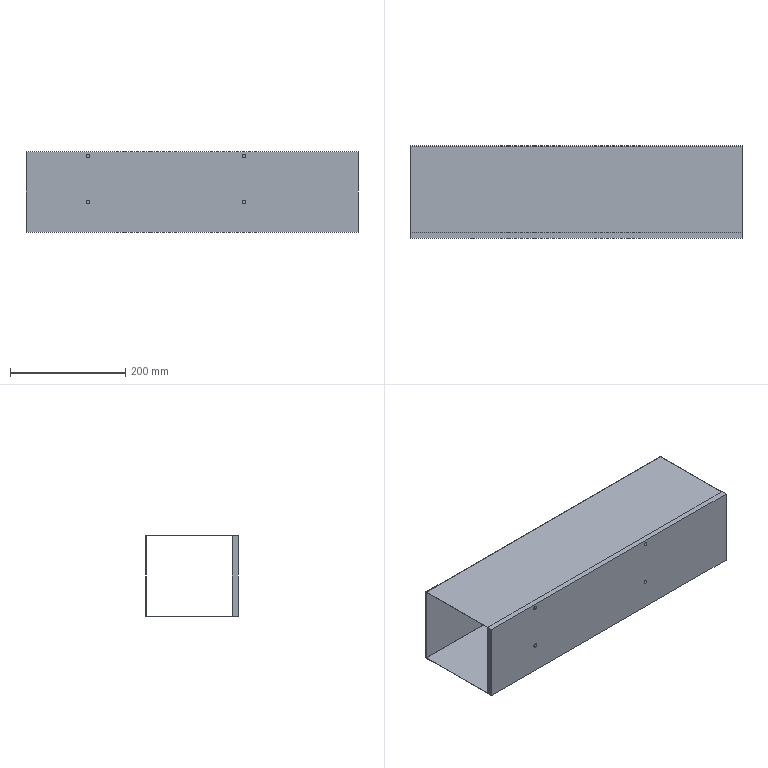Part | STEP file | 0245_Work-A | 1 solid | 18 faces | box 575 x 160 x 140 mm | volume 929885 mm3 | plane 10 | cylinder 8 | commonest cylinder face diameters 6.5 x8
STEP:
#1=CARTESIAN_POINT('',(0.,0.,0.));
#2=DIRECTION('',(0.,0.,1.));
#3=DIRECTION('',(1.,0.,0.));
#4=AXIS2_PLACEMENT_3D('',#1,#2,#3);
#5=CARTESIAN_POINT('',(377.5,0.,-84.25));
#6=VERTEX_POINT('',#5);
#7=CARTESIAN_POINT('',(377.5,10.,-84.25));
#8=VERTEX_POINT('',#7);
#9=CARTESIAN_POINT('',(377.5,10.,-84.25));
#10=DIRECTION('',(0.,1.,0.));
#11=VECTOR('',#10,1.);
#12=LINE('',#9,#11);
#13=CARTESIAN_POINT('',(377.5,10.,-87.5));
#14=DIRECTION('',(0.,1.,0.));
#15=DIRECTION('',(0.,0.,1.));
#16=AXIS2_PLACEMENT_3D('',#13,#14,#15);
#17=CYLINDRICAL_SURFACE('',#16,3.25);
#18=CARTESIAN_POINT('',(6.283,0.));
#19=DIRECTION('',(0.,1.));
#20=VECTOR('',#19,1.);
#21=LINE('',#18,#20);
#22=(GEOMETRIC_REPRESENTATION_CONTEXT(2)PARAMETRIC_REPRESENTATION_CONTEXT()REPRESENTATION_CONTEXT('',''));
#23=DEFINITIONAL_REPRESENTATION('',(#21),#22);
#24=PCURVE('',#17,#23);
#25=CARTESIAN_POINT('',(377.5,10.,-87.5));
#26=DIRECTION('',(0.,1.,0.));
#27=DIRECTION('',(0.,0.,1.));
#28=AXIS2_PLACEMENT_3D('',#25,#26,#27);
#29=CYLINDRICAL_SURFACE('',#28,3.25);
#30=CARTESIAN_POINT('',(0.,0.));
#31=DIRECTION('',(0.,1.));
#32=VECTOR('',#31,1.);
#33=LINE('',#30,#32);
#34=(GEOMETRIC_REPRESENTATION_CONTEXT(2)PARAMETRIC_REPRESENTATION_CONTEXT()REPRESENTATION_CONTEXT('',''));
#35=DEFINITIONAL_REPRESENTATION('',(#33),#34);
#36=PCURVE('',#29,#35);
#37=SURFACE_CURVE('',#12,(#24,#36),.PCURVE_S1.);
#38=EDGE_CURVE('',#6,#8,#37,.T.);
#39=ORIENTED_EDGE('',*,*,#38,.T.);
#40=CARTESIAN_POINT('',(377.5,10.,-90.75));
#41=VERTEX_POINT('',#40);
#42=CARTESIAN_POINT('',(377.5,10.,-87.5));
#43=DIRECTION('',(0.,1.,0.));
#44=DIRECTION('',(0.,0.,1.));
#45=AXIS2_PLACEMENT_3D('',#42,#43,#44);
#46=CIRCLE('',#45,3.25);
#47=CARTESIAN_POINT('',(0.,0.));
#48=DIRECTION('',(1.,0.));
#49=VECTOR('',#48,1.);
#50=LINE('',#47,#49);
#51=(GEOMETRIC_REPRESENTATION_CONTEXT(2)PARAMETRIC_REPRESENTATION_CONTEXT()REPRESENTATION_CONTEXT('',''));
#52=DEFINITIONAL_REPRESENTATION('',(#50),#51);
#53=PCURVE('',#17,#52);
#54=CARTESIAN_POINT('',(575.,10.,-0.5));
#55=DIRECTION('',(0.,1.,0.));
#56=DIRECTION('',(0.,0.,1.));
#57=AXIS2_PLACEMENT_3D('',#54,#55,#56);
#58=PLANE('',#57);
#59=CARTESIAN_POINT('',(-87.,-197.5));
#60=DIRECTION('',(1.,0.));
#61=AXIS2_PLACEMENT_2D('',#59,#60);
#62=CIRCLE('',#61,3.25);
#63=(GEOMETRIC_REPRESENTATION_CONTEXT(2)PARAMETRIC_REPRESENTATION_CONTEXT()REPRESENTATION_CONTEXT('',''));
#64=DEFINITIONAL_REPRESENTATION('',(#62),#63);
#65=PCURVE('',#58,#64);
#66=SURFACE_CURVE('',#46,(#53,#65),.PCURVE_S1.);
#67=EDGE_CURVE('',#41,#8,#66,.T.);
#68=ORIENTED_EDGE('',*,*,#67,.F.);
#69=CARTESIAN_POINT('',(377.5,0.,-90.75));
#70=VERTEX_POINT('',#69);
#71=CARTESIAN_POINT('',(377.5,10.,-90.75));
#72=DIRECTION('',(0.,1.,0.));
#73=VECTOR('',#72,1.);
#74=LINE('',#71,#73);
#75=CARTESIAN_POINT('',(3.142,0.));
#76=DIRECTION('',(0.,1.));
#77=VECTOR('',#76,1.);
#78=LINE('',#75,#77);
#79=(GEOMETRIC_REPRESENTATION_CONTEXT(2)PARAMETRIC_REPRESENTATION_CONTEXT()REPRESENTATION_CONTEXT('',''));
#80=DEFINITIONAL_REPRESENTATION('',(#78),#79);
#81=PCURVE('',#17,#80);
#82=CARTESIAN_POINT('',(3.142,0.));
#83=DIRECTION('',(0.,1.));
#84=VECTOR('',#83,1.);
#85=LINE('',#82,#84);
#86=(GEOMETRIC_REPRESENTATION_CONTEXT(2)PARAMETRIC_REPRESENTATION_CONTEXT()REPRESENTATION_CONTEXT('',''));
#87=DEFINITIONAL_REPRESENTATION('',(#85),#86);
#88=PCURVE('',#29,#87);
#89=SURFACE_CURVE('',#74,(#81,#88),.PCURVE_S1.);
#90=EDGE_CURVE('',#70,#41,#89,.T.);
#91=ORIENTED_EDGE('',*,*,#90,.F.);
#92=CARTESIAN_POINT('',(377.5,0.,-87.5));
#93=DIRECTION('',(0.,1.,0.));
#94=DIRECTION('',(0.,0.,1.));
#95=AXIS2_PLACEMENT_3D('',#92,#93,#94);
#96=CIRCLE('',#95,3.25);
#97=CARTESIAN_POINT('',(0.,-10.));
#98=DIRECTION('',(1.,0.));
#99=VECTOR('',#98,1.);
#100=LINE('',#97,#99);
#101=(GEOMETRIC_REPRESENTATION_CONTEXT(2)PARAMETRIC_REPRESENTATION_CONTEXT()REPRESENTATION_CONTEXT('',''));
#102=DEFINITIONAL_REPRESENTATION('',(#100),#101);
#103=PCURVE('',#17,#102);
#104=CARTESIAN_POINT('',(575.,0.,0.));
#105=DIRECTION('',(0.,1.,0.));
#106=DIRECTION('',(0.,0.,1.));
#107=AXIS2_PLACEMENT_3D('',#104,#105,#106);
#108=PLANE('',#107);
#109=CARTESIAN_POINT('',(-87.5,-197.5));
#110=DIRECTION('',(1.,0.));
#111=AXIS2_PLACEMENT_2D('',#109,#110);
#112=CIRCLE('',#111,3.25);
#113=(GEOMETRIC_REPRESENTATION_CONTEXT(2)PARAMETRIC_REPRESENTATION_CONTEXT()REPRESENTATION_CONTEXT('',''));
#114=DEFINITIONAL_REPRESENTATION('',(#112),#113);
#115=PCURVE('',#108,#114);
#116=SURFACE_CURVE('',#96,(#103,#115),.PCURVE_S1.);
#117=EDGE_CURVE('',#70,#6,#116,.T.);
#118=ORIENTED_EDGE('',*,*,#117,.T.);
#119=EDGE_LOOP('',(#39,#68,#91,#118));
#120=FACE_BOUND('',#119,.F.);
#121=ADVANCED_FACE('',(#120),#17,.F.);
#122=CARTESIAN_POINT('',(107.5,0.,-84.25));
#123=VERTEX_POINT('',#122);
#124=CARTESIAN_POINT('',(107.5,10.,-84.25));
#125=VERTEX_POINT('',#124);
#126=CARTESIAN_POINT('',(107.5,10.,-84.25));
#127=DIRECTION('',(0.,1.,0.));
#128=VECTOR('',#127,1.);
#129=LINE('',#126,#128);
#130=CARTESIAN_POINT('',(107.5,10.,-87.5));
#131=DIRECTION('',(0.,1.,0.));
#132=DIRECTION('',(0.,0.,1.));
#133=AXIS2_PLACEMENT_3D('',#130,#131,#132);
#134=CYLINDRICAL_SURFACE('',#133,3.25);
#135=CARTESIAN_POINT('',(6.283,0.));
#136=DIRECTION('',(0.,1.));
#137=VECTOR('',#136,1.);
#138=LINE('',#135,#137);
#139=(GEOMETRIC_REPRESENTATION_CONTEXT(2)PARAMETRIC_REPRESENTATION_CONTEXT()REPRESENTATION_CONTEXT('',''));
#140=DEFINITIONAL_REPRESENTATION('',(#138),#139);
#141=PCURVE('',#134,#140);
#142=CARTESIAN_POINT('',(107.5,10.,-87.5));
#143=DIRECTION('',(0.,1.,0.));
#144=DIRECTION('',(0.,0.,1.));
#145=AXIS2_PLACEMENT_3D('',#142,#143,#144);
#146=CYLINDRICAL_SURFACE('',#145,3.25);
#147=CARTESIAN_POINT('',(0.,0.));
#148=DIRECTION('',(0.,1.));
#149=VECTOR('',#148,1.);
#150=LINE('',#147,#149);
#151=(GEOMETRIC_REPRESENTATION_CONTEXT(2)PARAMETRIC_REPRESENTATION_CONTEXT()REPRESENTATION_CONTEXT('',''));
#152=DEFINITIONAL_REPRESENTATION('',(#150),#151);
#153=PCURVE('',#146,#152);
#154=SURFACE_CURVE('',#129,(#141,#153),.PCURVE_S1.);
#155=EDGE_CURVE('',#123,#125,#154,.T.);
#156=ORIENTED_EDGE('',*,*,#155,.T.);
#157=CARTESIAN_POINT('',(107.5,10.,-90.75));
#158=VERTEX_POINT('',#157);
#159=CARTESIAN_POINT('',(107.5,10.,-87.5));
#160=DIRECTION('',(0.,1.,0.));
#161=DIRECTION('',(0.,0.,1.));
#162=AXIS2_PLACEMENT_3D('',#159,#160,#161);
#163=CIRCLE('',#162,3.25);
#164=CARTESIAN_POINT('',(0.,0.));
#165=DIRECTION('',(1.,0.));
#166=VECTOR('',#165,1.);
#167=LINE('',#164,#166);
#168=(GEOMETRIC_REPRESENTATION_CONTEXT(2)PARAMETRIC_REPRESENTATION_CONTEXT()REPRESENTATION_CONTEXT('',''));
#169=DEFINITIONAL_REPRESENTATION('',(#167),#168);
#170=PCURVE('',#134,#169);
#171=CARTESIAN_POINT('',(-87.,-467.5));
#172=DIRECTION('',(1.,0.));
#173=AXIS2_PLACEMENT_2D('',#171,#172);
#174=CIRCLE('',#173,3.25);
#175=(GEOMETRIC_REPRESENTATION_CONTEXT(2)PARAMETRIC_REPRESENTATION_CONTEXT()REPRESENTATION_CONTEXT('',''));
#176=DEFINITIONAL_REPRESENTATION('',(#174),#175);
#177=PCURVE('',#58,#176);
#178=SURFACE_CURVE('',#163,(#170,#177),.PCURVE_S1.);
#179=EDGE_CURVE('',#158,#125,#178,.T.);
#180=ORIENTED_EDGE('',*,*,#179,.F.);
#181=CARTESIAN_POINT('',(107.5,0.,-90.75));
#182=VERTEX_POINT('',#181);
#183=CARTESIAN_POINT('',(107.5,10.,-90.75));
#184=DIRECTION('',(0.,1.,0.));
#185=VECTOR('',#184,1.);
#186=LINE('',#183,#185);
#187=CARTESIAN_POINT('',(3.142,0.));
#188=DIRECTION('',(0.,1.));
#189=VECTOR('',#188,1.);
#190=LINE('',#187,#189);
#191=(GEOMETRIC_REPRESENTATION_CONTEXT(2)PARAMETRIC_REPRESENTATION_CONTEXT()REPRESENTATION_CONTEXT('',''));
#192=DEFINITIONAL_REPRESENTATION('',(#190),#191);
#193=PCURVE('',#134,#192);
#194=CARTESIAN_POINT('',(3.142,0.));
#195=DIRECTION('',(0.,1.));
#196=VECTOR('',#195,1.);
#197=LINE('',#194,#196);
#198=(GEOMETRIC_REPRESENTATION_CONTEXT(2)PARAMETRIC_REPRESENTATION_CONTEXT()REPRESENTATION_CONTEXT('',''));
#199=DEFINITIONAL_REPRESENTATION('',(#197),#198);
#200=PCURVE('',#146,#199);
#201=SURFACE_CURVE('',#186,(#193,#200),.PCURVE_S1.);
#202=EDGE_CURVE('',#182,#158,#201,.T.);
#203=ORIENTED_EDGE('',*,*,#202,.F.);
#204=CARTESIAN_POINT('',(107.5,0.,-87.5));
#205=DIRECTION('',(0.,1.,0.));
#206=DIRECTION('',(0.,0.,1.));
#207=AXIS2_PLACEMENT_3D('',#204,#205,#206);
#208=CIRCLE('',#207,3.25);
#209=CARTESIAN_POINT('',(0.,-10.));
#210=DIRECTION('',(1.,0.));
#211=VECTOR('',#210,1.);
#212=LINE('',#209,#211);
#213=(GEOMETRIC_REPRESENTATION_CONTEXT(2)PARAMETRIC_REPRESENTATION_CONTEXT()REPRESENTATION_CONTEXT('',''));
#214=DEFINITIONAL_REPRESENTATION('',(#212),#213);
#215=PCURVE('',#134,#214);
#216=CARTESIAN_POINT('',(-87.5,-467.5));
#217=DIRECTION('',(1.,0.));
#218=AXIS2_PLACEMENT_2D('',#216,#217);
#219=CIRCLE('',#218,3.25);
#220=(GEOMETRIC_REPRESENTATION_CONTEXT(2)PARAMETRIC_REPRESENTATION_CONTEXT()REPRESENTATION_CONTEXT('',''));
#221=DEFINITIONAL_REPRESENTATION('',(#219),#220);
#222=PCURVE('',#108,#221);
#223=SURFACE_CURVE('',#208,(#215,#222),.PCURVE_S1.);
#224=EDGE_CURVE('',#182,#123,#223,.T.);
#225=ORIENTED_EDGE('',*,*,#224,.T.);
#226=EDGE_LOOP('',(#156,#180,#203,#225));
#227=FACE_BOUND('',#226,.F.);
#228=ADVANCED_FACE('',(#227),#134,.F.);
#229=CARTESIAN_POINT('',(377.5,0.,-4.25));
#230=VERTEX_POINT('',#229);
#231=CARTESIAN_POINT('',(377.5,10.,-4.25));
#232=VERTEX_POINT('',#231);
#233=CARTESIAN_POINT('',(377.5,10.,-4.25));
#234=DIRECTION('',(0.,1.,0.));
#235=VECTOR('',#234,1.);
#236=LINE('',#233,#235);
#237=CARTESIAN_POINT('',(377.5,10.,-7.5));
#238=DIRECTION('',(0.,1.,0.));
#239=DIRECTION('',(0.,0.,1.));
#240=AXIS2_PLACEMENT_3D('',#237,#238,#239);
#241=CYLINDRICAL_SURFACE('',#240,3.25);
#242=CARTESIAN_POINT('',(6.283,0.));
#243=DIRECTION('',(0.,1.));
#244=VECTOR('',#243,1.);
#245=LINE('',#242,#244);
#246=(GEOMETRIC_REPRESENTATION_CONTEXT(2)PARAMETRIC_REPRESENTATION_CONTEXT()REPRESENTATION_CONTEXT('',''));
#247=DEFINITIONAL_REPRESENTATION('',(#245),#246);
#248=PCURVE('',#241,#247);
#249=CARTESIAN_POINT('',(377.5,10.,-7.5));
#250=DIRECTION('',(0.,1.,0.));
#251=DIRECTION('',(0.,0.,1.));
#252=AXIS2_PLACEMENT_3D('',#249,#250,#251);
#253=CYLINDRICAL_SURFACE('',#252,3.25);
#254=CARTESIAN_POINT('',(0.,0.));
#255=DIRECTION('',(0.,1.));
#256=VECTOR('',#255,1.);
#257=LINE('',#254,#256);
#258=(GEOMETRIC_REPRESENTATION_CONTEXT(2)PARAMETRIC_REPRESENTATION_CONTEXT()REPRESENTATION_CONTEXT('',''));
#259=DEFINITIONAL_REPRESENTATION('',(#257),#258);
#260=PCURVE('',#253,#259);
#261=SURFACE_CURVE('',#236,(#248,#260),.PCURVE_S1.);
#262=EDGE_CURVE('',#230,#232,#261,.T.);
#263=ORIENTED_EDGE('',*,*,#262,.T.);
#264=CARTESIAN_POINT('',(377.5,10.,-10.75));
#265=VERTEX_POINT('',#264);
#266=CARTESIAN_POINT('',(377.5,10.,-7.5));
#267=DIRECTION('',(0.,1.,0.));
#268=DIRECTION('',(0.,0.,1.));
#269=AXIS2_PLACEMENT_3D('',#266,#267,#268);
#270=CIRCLE('',#269,3.25);
#271=CARTESIAN_POINT('',(0.,0.));
#272=DIRECTION('',(1.,0.));
#273=VECTOR('',#272,1.);
#274=LINE('',#271,#273);
#275=(GEOMETRIC_REPRESENTATION_CONTEXT(2)PARAMETRIC_REPRESENTATION_CONTEXT()REPRESENTATION_CONTEXT('',''));
#276=DEFINITIONAL_REPRESENTATION('',(#274),#275);
#277=PCURVE('',#241,#276);
#278=CARTESIAN_POINT('',(-7.,-197.5));
#279=DIRECTION('',(1.,0.));
#280=AXIS2_PLACEMENT_2D('',#278,#279);
#281=CIRCLE('',#280,3.25);
#282=(GEOMETRIC_REPRESENTATION_CONTEXT(2)PARAMETRIC_REPRESENTATION_CONTEXT()REPRESENTATION_CONTEXT('',''));
#283=DEFINITIONAL_REPRESENTATION('',(#281),#282);
#284=PCURVE('',#58,#283);
#285=SURFACE_CURVE('',#270,(#277,#284),.PCURVE_S1.);
#286=EDGE_CURVE('',#265,#232,#285,.T.);
#287=ORIENTED_EDGE('',*,*,#286,.F.);
#288=CARTESIAN_POINT('',(377.5,0.,-10.75));
#289=VERTEX_POINT('',#288);
#290=CARTESIAN_POINT('',(377.5,10.,-10.75));
#291=DIRECTION('',(0.,1.,0.));
#292=VECTOR('',#291,1.);
#293=LINE('',#290,#292);
#294=CARTESIAN_POINT('',(3.142,0.));
#295=DIRECTION('',(0.,1.));
#296=VECTOR('',#295,1.);
#297=LINE('',#294,#296);
#298=(GEOMETRIC_REPRESENTATION_CONTEXT(2)PARAMETRIC_REPRESENTATION_CONTEXT()REPRESENTATION_CONTEXT('',''));
#299=DEFINITIONAL_REPRESENTATION('',(#297),#298);
#300=PCURVE('',#241,#299);
#301=CARTESIAN_POINT('',(3.142,0.));
#302=DIRECTION('',(0.,1.));
#303=VECTOR('',#302,1.);
#304=LINE('',#301,#303);
#305=(GEOMETRIC_REPRESENTATION_CONTEXT(2)PARAMETRIC_REPRESENTATION_CONTEXT()REPRESENTATION_CONTEXT('',''));
#306=DEFINITIONAL_REPRESENTATION('',(#304),#305);
#307=PCURVE('',#253,#306);
#308=SURFACE_CURVE('',#293,(#300,#307),.PCURVE_S1.);
#309=EDGE_CURVE('',#289,#265,#308,.T.);
#310=ORIENTED_EDGE('',*,*,#309,.F.);
#311=CARTESIAN_POINT('',(377.5,0.,-7.5));
#312=DIRECTION('',(0.,1.,0.));
#313=DIRECTION('',(0.,0.,1.));
#314=AXIS2_PLACEMENT_3D('',#311,#312,#313);
#315=CIRCLE('',#314,3.25);
#316=CARTESIAN_POINT('',(0.,-10.));
#317=DIRECTION('',(1.,0.));
#318=VECTOR('',#317,1.);
#319=LINE('',#316,#318);
#320=(GEOMETRIC_REPRESENTATION_CONTEXT(2)PARAMETRIC_REPRESENTATION_CONTEXT()REPRESENTATION_CONTEXT('',''));
#321=DEFINITIONAL_REPRESENTATION('',(#319),#320);
#322=PCURVE('',#241,#321);
#323=CARTESIAN_POINT('',(-7.5,-197.5));
#324=DIRECTION('',(1.,0.));
#325=AXIS2_PLACEMENT_2D('',#323,#324);
#326=CIRCLE('',#325,3.25);
#327=(GEOMETRIC_REPRESENTATION_CONTEXT(2)PARAMETRIC_REPRESENTATION_CONTEXT()REPRESENTATION_CONTEXT('',''));
#328=DEFINITIONAL_REPRESENTATION('',(#326),#327);
#329=PCURVE('',#108,#328);
#330=SURFACE_CURVE('',#315,(#322,#329),.PCURVE_S1.);
#331=EDGE_CURVE('',#289,#230,#330,.T.);
#332=ORIENTED_EDGE('',*,*,#331,.T.);
#333=EDGE_LOOP('',(#263,#287,#310,#332));
#334=FACE_BOUND('',#333,.F.);
#335=ADVANCED_FACE('',(#334),#241,.F.);
#336=CARTESIAN_POINT('',(107.5,0.,-4.25));
#337=VERTEX_POINT('',#336);
#338=CARTESIAN_POINT('',(107.5,10.,-4.25));
#339=VERTEX_POINT('',#338);
#340=CARTESIAN_POINT('',(107.5,10.,-4.25));
#341=DIRECTION('',(0.,1.,0.));
#342=VECTOR('',#341,1.);
#343=LINE('',#340,#342);
#344=CARTESIAN_POINT('',(107.5,10.,-7.5));
#345=DIRECTION('',(0.,1.,0.));
#346=DIRECTION('',(0.,0.,1.));
#347=AXIS2_PLACEMENT_3D('',#344,#345,#346);
#348=CYLINDRICAL_SURFACE('',#347,3.25);
#349=CARTESIAN_POINT('',(6.283,0.));
#350=DIRECTION('',(0.,1.));
#351=VECTOR('',#350,1.);
#352=LINE('',#349,#351);
#353=(GEOMETRIC_REPRESENTATION_CONTEXT(2)PARAMETRIC_REPRESENTATION_CONTEXT()REPRESENTATION_CONTEXT('',''));
#354=DEFINITIONAL_REPRESENTATION('',(#352),#353);
#355=PCURVE('',#348,#354);
#356=CARTESIAN_POINT('',(107.5,10.,-7.5));
#357=DIRECTION('',(0.,1.,0.));
#358=DIRECTION('',(0.,0.,1.));
#359=AXIS2_PLACEMENT_3D('',#356,#357,#358);
#360=CYLINDRICAL_SURFACE('',#359,3.25);
#361=CARTESIAN_POINT('',(0.,0.));
#362=DIRECTION('',(0.,1.));
#363=VECTOR('',#362,1.);
#364=LINE('',#361,#363);
#365=(GEOMETRIC_REPRESENTATION_CONTEXT(2)PARAMETRIC_REPRESENTATION_CONTEXT()REPRESENTATION_CONTEXT('',''));
#366=DEFINITIONAL_REPRESENTATION('',(#364),#365);
#367=PCURVE('',#360,#366);
#368=SURFACE_CURVE('',#343,(#355,#367),.PCURVE_S1.);
#369=EDGE_CURVE('',#337,#339,#368,.T.);
#370=ORIENTED_EDGE('',*,*,#369,.T.);
#371=CARTESIAN_POINT('',(107.5,10.,-10.75));
#372=VERTEX_POINT('',#371);
#373=CARTESIAN_POINT('',(107.5,10.,-7.5));
#374=DIRECTION('',(0.,1.,0.));
#375=DIRECTION('',(0.,0.,1.));
#376=AXIS2_PLACEMENT_3D('',#373,#374,#375);
#377=CIRCLE('',#376,3.25);
#378=CARTESIAN_POINT('',(0.,0.));
#379=DIRECTION('',(1.,0.));
#380=VECTOR('',#379,1.);
#381=LINE('',#378,#380);
#382=(GEOMETRIC_REPRESENTATION_CONTEXT(2)PARAMETRIC_REPRESENTATION_CONTEXT()REPRESENTATION_CONTEXT('',''));
#383=DEFINITIONAL_REPRESENTATION('',(#381),#382);
#384=PCURVE('',#348,#383);
#385=CARTESIAN_POINT('',(-7.,-467.5));
#386=DIRECTION('',(1.,0.));
#387=AXIS2_PLACEMENT_2D('',#385,#386);
#388=CIRCLE('',#387,3.25);
#389=(GEOMETRIC_REPRESENTATION_CONTEXT(2)PARAMETRIC_REPRESENTATION_CONTEXT()REPRESENTATION_CONTEXT('',''));
#390=DEFINITIONAL_REPRESENTATION('',(#388),#389);
#391=PCURVE('',#58,#390);
#392=SURFACE_CURVE('',#377,(#384,#391),.PCURVE_S1.);
#393=EDGE_CURVE('',#372,#339,#392,.T.);
#394=ORIENTED_EDGE('',*,*,#393,.F.);
#395=CARTESIAN_POINT('',(107.5,0.,-10.75));
#396=VERTEX_POINT('',#395);
#397=CARTESIAN_POINT('',(107.5,10.,-10.75));
#398=DIRECTION('',(0.,1.,0.));
#399=VECTOR('',#398,1.);
#400=LINE('',#397,#399);
#401=CARTESIAN_POINT('',(3.142,0.));
#402=DIRECTION('',(0.,1.));
#403=VECTOR('',#402,1.);
#404=LINE('',#401,#403);
#405=(GEOMETRIC_REPRESENTATION_CONTEXT(2)PARAMETRIC_REPRESENTATION_CONTEXT()REPRESENTATION_CONTEXT('',''));
#406=DEFINITIONAL_REPRESENTATION('',(#404),#405);
#407=PCURVE('',#348,#406);
#408=CARTESIAN_POINT('',(3.142,0.));
#409=DIRECTION('',(0.,1.));
#410=VECTOR('',#409,1.);
#411=LINE('',#408,#410);
#412=(GEOMETRIC_REPRESENTATION_CONTEXT(2)PARAMETRIC_REPRESENTATION_CONTEXT()REPRESENTATION_CONTEXT('',''));
#413=DEFINITIONAL_REPRESENTATION('',(#411),#412);
#414=PCURVE('',#360,#413);
#415=SURFACE_CURVE('',#400,(#407,#414),.PCURVE_S1.);
#416=EDGE_CURVE('',#396,#372,#415,.T.);
#417=ORIENTED_EDGE('',*,*,#416,.F.);
#418=CARTESIAN_POINT('',(107.5,0.,-7.5));
#419=DIRECTION('',(0.,1.,0.));
#420=DIRECTION('',(0.,0.,1.));
#421=AXIS2_PLACEMENT_3D('',#418,#419,#420);
#422=CIRCLE('',#421,3.25);
#423=CARTESIAN_POINT('',(0.,-10.));
#424=DIRECTION('',(1.,0.));
#425=VECTOR('',#424,1.);
#426=LINE('',#423,#425);
#427=(GEOMETRIC_REPRESENTATION_CONTEXT(2)PARAMETRIC_REPRESENTATION_CONTEXT()REPRESENTATION_CONTEXT('',''));
#428=DEFINITIONAL_REPRESENTATION('',(#426),#427);
#429=PCURVE('',#348,#428);
#430=CARTESIAN_POINT('',(-7.5,-467.5));
#431=DIRECTION('',(1.,0.));
#432=AXIS2_PLACEMENT_2D('',#430,#431);
#433=CIRCLE('',#432,3.25);
#434=(GEOMETRIC_REPRESENTATION_CONTEXT(2)PARAMETRIC_REPRESENTATION_CONTEXT()REPRESENTATION_CONTEXT('',''));
#435=DEFINITIONAL_REPRESENTATION('',(#433),#434);
#436=PCURVE('',#108,#435);
#437=SURFACE_CURVE('',#422,(#429,#436),.PCURVE_S1.);
#438=EDGE_CURVE('',#396,#337,#437,.T.);
#439=ORIENTED_EDGE('',*,*,#438,.T.);
#440=EDGE_LOOP('',(#370,#394,#417,#439));
#441=FACE_BOUND('',#440,.F.);
#442=ADVANCED_FACE('',(#441),#348,.F.);
#443=CARTESIAN_POINT('',(575.,160.,0.));
#444=VERTEX_POINT('',#443);
#445=CARTESIAN_POINT('',(575.,0.,0.));
#446=VERTEX_POINT('',#445);
#447=CARTESIAN_POINT('',(575.,0.,0.));
#448=DIRECTION('',(0.,-1.,0.));
#449=VECTOR('',#448,1.);
#450=LINE('',#447,#449);
#451=CARTESIAN_POINT('',(575.,160.,0.));
#452=DIRECTION('',(-1.,0.,0.));
#453=DIRECTION('',(0.,0.,1.));
#454=AXIS2_PLACEMENT_3D('',#451,#452,#453);
#455=PLANE('',#454);
#456=CARTESIAN_POINT('',(0.,-160.));
#457=DIRECTION('',(0.,-1.));
#458=VECTOR('',#457,1.);
#459=LINE('',#456,#458);
#460=(GEOMETRIC_REPRESENTATION_CONTEXT(2)PARAMETRIC_REPRESENTATION_CONTEXT()REPRESENTATION_CONTEXT('',''));
#461=DEFINITIONAL_REPRESENTATION('',(#459),#460);
#462=PCURVE('',#455,#461);
#463=CARTESIAN_POINT('',(575.,0.,0.));
#464=DIRECTION('',(0.,0.,-1.));
#465=DIRECTION('',(-1.,0.,0.));
#466=AXIS2_PLACEMENT_3D('',#463,#464,#465);
#467=PLANE('',#466);
#468=CARTESIAN_POINT('',(0.,0.));
#469=DIRECTION('',(0.,-1.));
#470=VECTOR('',#469,1.);
#471=LINE('',#468,#470);
#472=(GEOMETRIC_REPRESENTATION_CONTEXT(2)PARAMETRIC_REPRESENTATION_CONTEXT()REPRESENTATION_CONTEXT('',''));
#473=DEFINITIONAL_REPRESENTATION('',(#471),#472);
#474=PCURVE('',#467,#473);
#475=SURFACE_CURVE('',#450,(#462,#474),.PCURVE_S1.);
#476=EDGE_CURVE('',#444,#446,#475,.T.);
#477=ORIENTED_EDGE('',*,*,#476,.T.);
#478=CARTESIAN_POINT('',(575.,0.,-140.));
#479=VERTEX_POINT('',#478);
#480=CARTESIAN_POINT('',(575.,0.,0.));
#481=DIRECTION('',(0.,0.,-1.));
#482=VECTOR('',#481,1.);
#483=LINE('',#480,#482);
#484=CARTESIAN_POINT('',(0.,-160.));
#485=DIRECTION('',(-1.,0.));
#486=VECTOR('',#485,1.);
#487=LINE('',#484,#486);
#488=(GEOMETRIC_REPRESENTATION_CONTEXT(2)PARAMETRIC_REPRESENTATION_CONTEXT()REPRESENTATION_CONTEXT('',''));
#489=DEFINITIONAL_REPRESENTATION('',(#487),#488);
#490=PCURVE('',#455,#489);
#491=CARTESIAN_POINT('',(0.,0.));
#492=DIRECTION('',(-1.,0.));
#493=VECTOR('',#492,1.);
#494=LINE('',#491,#493);
#495=(GEOMETRIC_REPRESENTATION_CONTEXT(2)PARAMETRIC_REPRESENTATION_CONTEXT()REPRESENTATION_CONTEXT('',''));
#496=DEFINITIONAL_REPRESENTATION('',(#494),#495);
#497=PCURVE('',#108,#496);
#498=SURFACE_CURVE('',#483,(#490,#497),.PCURVE_S1.);
#499=EDGE_CURVE('',#446,#479,#498,.T.);
#500=ORIENTED_EDGE('',*,*,#499,.T.);
#501=CARTESIAN_POINT('',(575.,160.,-140.));
#502=VERTEX_POINT('',#501);
#503=CARTESIAN_POINT('',(575.,0.,-140.));
#504=DIRECTION('',(0.,1.,0.));
#505=VECTOR('',#504,1.);
#506=LINE('',#503,#505);
#507=CARTESIAN_POINT('',(-140.,-160.));
#508=DIRECTION('',(0.,1.));
#509=VECTOR('',#508,1.);
#510=LINE('',#507,#509);
#511=(GEOMETRIC_REPRESENTATION_CONTEXT(2)PARAMETRIC_REPRESENTATION_CONTEXT()REPRESENTATION_CONTEXT('',''));
#512=DEFINITIONAL_REPRESENTATION('',(#510),#511);
#513=PCURVE('',#455,#512);
#514=CARTESIAN_POINT('',(575.,0.,-140.));
#515=DIRECTION('',(0.,0.,1.));
#516=DIRECTION('',(1.,0.,0.));
#517=AXIS2_PLACEMENT_3D('',#514,#515,#516);
#518=PLANE('',#517);
#519=CARTESIAN_POINT('',(0.,0.));
#520=DIRECTION('',(0.,1.));
#521=VECTOR('',#520,1.);
#522=LINE('',#519,#521);
#523=(GEOMETRIC_REPRESENTATION_CONTEXT(2)PARAMETRIC_REPRESENTATION_CONTEXT()REPRESENTATION_CONTEXT('',''));
#524=DEFINITIONAL_REPRESENTATION('',(#522),#523);
#525=PCURVE('',#518,#524);
#526=SURFACE_CURVE('',#506,(#513,#525),.PCURVE_S1.);
#527=EDGE_CURVE('',#479,#502,#526,.T.);
#528=ORIENTED_EDGE('',*,*,#527,.T.);
#529=CARTESIAN_POINT('',(575.,160.,0.));
#530=DIRECTION('',(0.,0.,1.));
#531=VECTOR('',#530,1.);
#532=LINE('',#529,#531);
#533=CARTESIAN_POINT('',(0.,0.));
#534=DIRECTION('',(1.,0.));
#535=VECTOR('',#534,1.);
#536=LINE('',#533,#535);
#537=(GEOMETRIC_REPRESENTATION_CONTEXT(2)PARAMETRIC_REPRESENTATION_CONTEXT()REPRESENTATION_CONTEXT('',''));
#538=DEFINITIONAL_REPRESENTATION('',(#536),#537);
#539=PCURVE('',#455,#538);
#540=CARTESIAN_POINT('',(575.,160.,0.));
#541=DIRECTION('',(0.,-1.,0.));
#542=DIRECTION('',(0.,0.,-1.));
#543=AXIS2_PLACEMENT_3D('',#540,#541,#542);
#544=PLANE('',#543);
#545=CARTESIAN_POINT('',(0.,0.));
#546=DIRECTION('',(-1.,0.));
#547=VECTOR('',#546,1.);
#548=LINE('',#545,#547);
#549=(GEOMETRIC_REPRESENTATION_CONTEXT(2)PARAMETRIC_REPRESENTATION_CONTEXT()REPRESENTATION_CONTEXT('',''));
#550=DEFINITIONAL_REPRESENTATION('',(#548),#549);
#551=PCURVE('',#544,#550);
#552=SURFACE_CURVE('',#532,(#539,#551),.PCURVE_S1.);
#553=EDGE_CURVE('',#502,#444,#552,.T.);
#554=ORIENTED_EDGE('',*,*,#553,.T.);
#555=EDGE_LOOP('',(#477,#500,#528,#554));
#556=FACE_BOUND('',#555,.T.);
#557=CARTESIAN_POINT('',(575.,159.5,-0.5));
#558=VERTEX_POINT('',#557);
#559=CARTESIAN_POINT('',(575.,10.,-0.5));
#560=VERTEX_POINT('',#559);
#561=CARTESIAN_POINT('',(575.,10.,-0.5));
#562=DIRECTION('',(0.,-1.,0.));
#563=VECTOR('',#562,1.);
#564=LINE('',#561,#563);
#565=CARTESIAN_POINT('',(-0.5,-150.));
#566=DIRECTION('',(0.,-1.));
#567=VECTOR('',#566,1.);
#568=LINE('',#565,#567);
#569=(GEOMETRIC_REPRESENTATION_CONTEXT(2)PARAMETRIC_REPRESENTATION_CONTEXT()REPRESENTATION_CONTEXT('',''));
#570=DEFINITIONAL_REPRESENTATION('',(#568),#569);
#571=PCURVE('',#455,#570);
#572=CARTESIAN_POINT('',(575.,10.,-0.5));
#573=DIRECTION('',(0.,0.,-1.));
#574=DIRECTION('',(-1.,0.,0.));
#575=AXIS2_PLACEMENT_3D('',#572,#573,#574);
#576=PLANE('',#575);
#577=CARTESIAN_POINT('',(0.,0.));
#578=DIRECTION('',(0.,-1.));
#579=VECTOR('',#578,1.);
#580=LINE('',#577,#579);
#581=(GEOMETRIC_REPRESENTATION_CONTEXT(2)PARAMETRIC_REPRESENTATION_CONTEXT()REPRESENTATION_CONTEXT('',''));
#582=DEFINITIONAL_REPRESENTATION('',(#580),#581);
#583=PCURVE('',#576,#582);
#584=SURFACE_CURVE('',#564,(#571,#583),.PCURVE_S1.);
#585=EDGE_CURVE('',#558,#560,#584,.T.);
#586=ORIENTED_EDGE('',*,*,#585,.F.);
#587=CARTESIAN_POINT('',(575.,159.5,-139.5));
#588=VERTEX_POINT('',#587);
#589=CARTESIAN_POINT('',(575.,159.5,-0.5));
#590=DIRECTION('',(0.,0.,1.));
#591=VECTOR('',#590,1.);
#592=LINE('',#589,#591);
#593=CARTESIAN_POINT('',(-0.5,-0.5));
#594=DIRECTION('',(1.,0.));
#595=VECTOR('',#594,1.);
#596=LINE('',#593,#595);
#597=(GEOMETRIC_REPRESENTATION_CONTEXT(2)PARAMETRIC_REPRESENTATION_CONTEXT()REPRESENTATION_CONTEXT('',''));
#598=DEFINITIONAL_REPRESENTATION('',(#596),#597);
#599=PCURVE('',#455,#598);
#600=CARTESIAN_POINT('',(575.,159.5,-0.5));
#601=DIRECTION('',(0.,-1.,0.));
#602=DIRECTION('',(0.,0.,-1.));
#603=AXIS2_PLACEMENT_3D('',#600,#601,#602);
#604=PLANE('',#603);
#605=CARTESIAN_POINT('',(0.,0.));
#606=DIRECTION('',(-1.,0.));
#607=VECTOR('',#606,1.);
#608=LINE('',#605,#607);
#609=(GEOMETRIC_REPRESENTATION_CONTEXT(2)PARAMETRIC_REPRESENTATION_CONTEXT()REPRESENTATION_CONTEXT('',''));
#610=DEFINITIONAL_REPRESENTATION('',(#608),#609);
#611=PCURVE('',#604,#610);
#612=SURFACE_CURVE('',#592,(#599,#611),.PCURVE_S1.);
#613=EDGE_CURVE('',#588,#558,#612,.T.);
#614=ORIENTED_EDGE('',*,*,#613,.F.);
#615=CARTESIAN_POINT('',(575.,10.,-139.5));
#616=VERTEX_POINT('',#615);
#617=CARTESIAN_POINT('',(575.,10.,-139.5));
#618=DIRECTION('',(0.,1.,0.));
#619=VECTOR('',#618,1.);
#620=LINE('',#617,#619);
#621=CARTESIAN_POINT('',(-139.5,-150.));
#622=DIRECTION('',(0.,1.));
#623=VECTOR('',#622,1.);
#624=LINE('',#621,#623);
#625=(GEOMETRIC_REPRESENTATION_CONTEXT(2)PARAMETRIC_REPRESENTATION_CONTEXT()REPRESENTATION_CONTEXT('',''));
#626=DEFINITIONAL_REPRESENTATION('',(#624),#625);
#627=PCURVE('',#455,#626);
#628=CARTESIAN_POINT('',(575.,10.,-139.5));
#629=DIRECTION('',(0.,0.,1.));
#630=DIRECTION('',(1.,0.,0.));
#631=AXIS2_PLACEMENT_3D('',#628,#629,#630);
#632=PLANE('',#631);
#633=CARTESIAN_POINT('',(0.,0.));
#634=DIRECTION('',(0.,1.));
#635=VECTOR('',#634,1.);
#636=LINE('',#633,#635);
#637=(GEOMETRIC_REPRESENTATION_CONTEXT(2)PARAMETRIC_REPRESENTATION_CONTEXT()REPRESENTATION_CONTEXT('',''));
#638=DEFINITIONAL_REPRESENTATION('',(#636),#637);
#639=PCURVE('',#632,#638);
#640=SURFACE_CURVE('',#620,(#627,#639),.PCURVE_S1.);
#641=EDGE_CURVE('',#616,#588,#640,.T.);
#642=ORIENTED_EDGE('',*,*,#641,.F.);
#643=CARTESIAN_POINT('',(575.,10.,-0.5));
#644=DIRECTION('',(0.,0.,-1.));
#645=VECTOR('',#644,1.);
#646=LINE('',#643,#645);
#647=CARTESIAN_POINT('',(-0.5,-150.));
#648=DIRECTION('',(-1.,0.));
#649=VECTOR('',#648,1.);
#650=LINE('',#647,#649);
#651=(GEOMETRIC_REPRESENTATION_CONTEXT(2)PARAMETRIC_REPRESENTATION_CONTEXT()REPRESENTATION_CONTEXT('',''));
#652=DEFINITIONAL_REPRESENTATION('',(#650),#651);
#653=PCURVE('',#455,#652);
#654=CARTESIAN_POINT('',(0.,0.));
#655=DIRECTION('',(-1.,0.));
#656=VECTOR('',#655,1.);
#657=LINE('',#654,#656);
#658=(GEOMETRIC_REPRESENTATION_CONTEXT(2)PARAMETRIC_REPRESENTATION_CONTEXT()REPRESENTATION_CONTEXT('',''));
#659=DEFINITIONAL_REPRESENTATION('',(#657),#658);
#660=PCURVE('',#58,#659);
#661=SURFACE_CURVE('',#646,(#653,#660),.PCURVE_S1.);
#662=EDGE_CURVE('',#560,#616,#661,.T.);
#663=ORIENTED_EDGE('',*,*,#662,.F.);
#664=EDGE_LOOP('',(#586,#614,#642,#663));
#665=FACE_BOUND('',#664,.T.);
#666=ADVANCED_FACE('',(#556,#665),#455,.F.);
#667=CARTESIAN_POINT('',(0.,160.,0.));
#668=VERTEX_POINT('',#667);
#669=CARTESIAN_POINT('',(0.,0.,0.));
#670=VERTEX_POINT('',#669);
#671=CARTESIAN_POINT('',(0.,0.,0.));
#672=DIRECTION('',(0.,-1.,0.));
#673=VECTOR('',#672,1.);
#674=LINE('',#671,#673);
#675=CARTESIAN_POINT('',(0.,160.,0.));
#676=DIRECTION('',(-1.,0.,0.));
#677=DIRECTION('',(0.,0.,1.));
#678=AXIS2_PLACEMENT_3D('',#675,#676,#677);
#679=PLANE('',#678);
#680=CARTESIAN_POINT('',(0.,-160.));
#681=DIRECTION('',(0.,-1.));
#682=VECTOR('',#681,1.);
#683=LINE('',#680,#682);
#684=(GEOMETRIC_REPRESENTATION_CONTEXT(2)PARAMETRIC_REPRESENTATION_CONTEXT()REPRESENTATION_CONTEXT('',''));
#685=DEFINITIONAL_REPRESENTATION('',(#683),#684);
#686=PCURVE('',#679,#685);
#687=CARTESIAN_POINT('',(575.,0.));
#688=DIRECTION('',(0.,-1.));
#689=VECTOR('',#688,1.);
#690=LINE('',#687,#689);
#691=(GEOMETRIC_REPRESENTATION_CONTEXT(2)PARAMETRIC_REPRESENTATION_CONTEXT()REPRESENTATION_CONTEXT('',''));
#692=DEFINITIONAL_REPRESENTATION('',(#690),#691);
#693=PCURVE('',#467,#692);
#694=SURFACE_CURVE('',#674,(#686,#693),.PCURVE_S1.);
#695=EDGE_CURVE('',#668,#670,#694,.T.);
#696=ORIENTED_EDGE('',*,*,#695,.F.);
#697=CARTESIAN_POINT('',(0.,160.,-140.));
#698=VERTEX_POINT('',#697);
#699=CARTESIAN_POINT('',(0.,160.,0.));
#700=DIRECTION('',(0.,0.,1.));
#701=VECTOR('',#700,1.);
#702=LINE('',#699,#701);
#703=CARTESIAN_POINT('',(0.,0.));
#704=DIRECTION('',(1.,0.));
#705=VECTOR('',#704,1.);
#706=LINE('',#703,#705);
#707=(GEOMETRIC_REPRESENTATION_CONTEXT(2)PARAMETRIC_REPRESENTATION_CONTEXT()REPRESENTATION_CONTEXT('',''));
#708=DEFINITIONAL_REPRESENTATION('',(#706),#707);
#709=PCURVE('',#679,#708);
#710=CARTESIAN_POINT('',(0.,-575.));
#711=DIRECTION('',(-1.,0.));
#712=VECTOR('',#711,1.);
#713=LINE('',#710,#712);
#714=(GEOMETRIC_REPRESENTATION_CONTEXT(2)PARAMETRIC_REPRESENTATION_CONTEXT()REPRESENTATION_CONTEXT('',''));
#715=DEFINITIONAL_REPRESENTATION('',(#713),#714);
#716=PCURVE('',#544,#715);
#717=SURFACE_CURVE('',#702,(#709,#716),.PCURVE_S1.);
#718=EDGE_CURVE('',#698,#668,#717,.T.);
#719=ORIENTED_EDGE('',*,*,#718,.F.);
#720=CARTESIAN_POINT('',(0.,0.,-140.));
#721=VERTEX_POINT('',#720);
#722=CARTESIAN_POINT('',(0.,0.,-140.));
#723=DIRECTION('',(0.,1.,0.));
#724=VECTOR('',#723,1.);
#725=LINE('',#722,#724);
#726=CARTESIAN_POINT('',(-140.,-160.));
#727=DIRECTION('',(0.,1.));
#728=VECTOR('',#727,1.);
#729=LINE('',#726,#728);
#730=(GEOMETRIC_REPRESENTATION_CONTEXT(2)PARAMETRIC_REPRESENTATION_CONTEXT()REPRESENTATION_CONTEXT('',''));
#731=DEFINITIONAL_REPRESENTATION('',(#729),#730);
#732=PCURVE('',#679,#731);
#733=CARTESIAN_POINT('',(-575.,0.));
#734=DIRECTION('',(0.,1.));
#735=VECTOR('',#734,1.);
#736=LINE('',#733,#735);
#737=(GEOMETRIC_REPRESENTATION_CONTEXT(2)PARAMETRIC_REPRESENTATION_CONTEXT()REPRESENTATION_CONTEXT('',''));
#738=DEFINITIONAL_REPRESENTATION('',(#736),#737);
#739=PCURVE('',#518,#738);
#740=SURFACE_CURVE('',#725,(#732,#739),.PCURVE_S1.);
#741=EDGE_CURVE('',#721,#698,#740,.T.);
#742=ORIENTED_EDGE('',*,*,#741,.F.);
#743=CARTESIAN_POINT('',(0.,0.,0.));
#744=DIRECTION('',(0.,0.,-1.));
#745=VECTOR('',#744,1.);
#746=LINE('',#743,#745);
#747=CARTESIAN_POINT('',(0.,-160.));
#748=DIRECTION('',(-1.,0.));
#749=VECTOR('',#748,1.);
#750=LINE('',#747,#749);
#751=(GEOMETRIC_REPRESENTATION_CONTEXT(2)PARAMETRIC_REPRESENTATION_CONTEXT()REPRESENTATION_CONTEXT('',''));
#752=DEFINITIONAL_REPRESENTATION('',(#750),#751);
#753=PCURVE('',#679,#752);
#754=CARTESIAN_POINT('',(0.,-575.));
#755=DIRECTION('',(-1.,0.));
#756=VECTOR('',#755,1.);
#757=LINE('',#754,#756);
#758=(GEOMETRIC_REPRESENTATION_CONTEXT(2)PARAMETRIC_REPRESENTATION_CONTEXT()REPRESENTATION_CONTEXT('',''));
#759=DEFINITIONAL_REPRESENTATION('',(#757),#758);
#760=PCURVE('',#108,#759);
#761=SURFACE_CURVE('',#746,(#753,#760),.PCURVE_S1.);
#762=EDGE_CURVE('',#670,#721,#761,.T.);
#763=ORIENTED_EDGE('',*,*,#762,.F.);
#764=EDGE_LOOP('',(#696,#719,#742,#763));
#765=FACE_BOUND('',#764,.T.);
#766=CARTESIAN_POINT('',(0.,159.5,-139.5));
#767=VERTEX_POINT('',#766);
#768=CARTESIAN_POINT('',(0.,159.5,-0.5));
#769=VERTEX_POINT('',#768);
#770=CARTESIAN_POINT('',(0.,159.5,-0.5));
#771=DIRECTION('',(0.,0.,1.));
#772=VECTOR('',#771,1.);
#773=LINE('',#770,#772);
#774=CARTESIAN_POINT('',(-0.5,-0.5));
#775=DIRECTION('',(1.,0.));
#776=VECTOR('',#775,1.);
#777=LINE('',#774,#776);
#778=(GEOMETRIC_REPRESENTATION_CONTEXT(2)PARAMETRIC_REPRESENTATION_CONTEXT()REPRESENTATION_CONTEXT('',''));
#779=DEFINITIONAL_REPRESENTATION('',(#777),#778);
#780=PCURVE('',#679,#779);
#781=CARTESIAN_POINT('',(0.,-575.));
#782=DIRECTION('',(-1.,0.));
#783=VECTOR('',#782,1.);
#784=LINE('',#781,#783);
#785=(GEOMETRIC_REPRESENTATION_CONTEXT(2)PARAMETRIC_REPRESENTATION_CONTEXT()REPRESENTATION_CONTEXT('',''));
#786=DEFINITIONAL_REPRESENTATION('',(#784),#785);
#787=PCURVE('',#604,#786);
#788=SURFACE_CURVE('',#773,(#780,#787),.PCURVE_S1.);
#789=EDGE_CURVE('',#767,#769,#788,.T.);
#790=ORIENTED_EDGE('',*,*,#789,.T.);
#791=CARTESIAN_POINT('',(0.,10.,-0.5));
#792=VERTEX_POINT('',#791);
#793=CARTESIAN_POINT('',(0.,10.,-0.5));
#794=DIRECTION('',(0.,-1.,0.));
#795=VECTOR('',#794,1.);
#796=LINE('',#793,#795);
#797=CARTESIAN_POINT('',(-0.5,-150.));
#798=DIRECTION('',(0.,-1.));
#799=VECTOR('',#798,1.);
#800=LINE('',#797,#799);
#801=(GEOMETRIC_REPRESENTATION_CONTEXT(2)PARAMETRIC_REPRESENTATION_CONTEXT()REPRESENTATION_CONTEXT('',''));
#802=DEFINITIONAL_REPRESENTATION('',(#800),#801);
#803=PCURVE('',#679,#802);
#804=CARTESIAN_POINT('',(575.,0.));
#805=DIRECTION('',(0.,-1.));
#806=VECTOR('',#805,1.);
#807=LINE('',#804,#806);
#808=(GEOMETRIC_REPRESENTATION_CONTEXT(2)PARAMETRIC_REPRESENTATION_CONTEXT()REPRESENTATION_CONTEXT('',''));
#809=DEFINITIONAL_REPRESENTATION('',(#807),#808);
#810=PCURVE('',#576,#809);
#811=SURFACE_CURVE('',#796,(#803,#810),.PCURVE_S1.);
#812=EDGE_CURVE('',#769,#792,#811,.T.);
#813=ORIENTED_EDGE('',*,*,#812,.T.);
#814=CARTESIAN_POINT('',(0.,10.,-139.5));
#815=VERTEX_POINT('',#814);
#816=CARTESIAN_POINT('',(0.,10.,-0.5));
#817=DIRECTION('',(0.,0.,-1.));
#818=VECTOR('',#817,1.);
#819=LINE('',#816,#818);
#820=CARTESIAN_POINT('',(-0.5,-150.));
#821=DIRECTION('',(-1.,0.));
#822=VECTOR('',#821,1.);
#823=LINE('',#820,#822);
#824=(GEOMETRIC_REPRESENTATION_CONTEXT(2)PARAMETRIC_REPRESENTATION_CONTEXT()REPRESENTATION_CONTEXT('',''));
#825=DEFINITIONAL_REPRESENTATION('',(#823),#824);
#826=PCURVE('',#679,#825);
#827=CARTESIAN_POINT('',(0.,-575.));
#828=DIRECTION('',(-1.,0.));
#829=VECTOR('',#828,1.);
#830=LINE('',#827,#829);
#831=(GEOMETRIC_REPRESENTATION_CONTEXT(2)PARAMETRIC_REPRESENTATION_CONTEXT()REPRESENTATION_CONTEXT('',''));
#832=DEFINITIONAL_REPRESENTATION('',(#830),#831);
#833=PCURVE('',#58,#832);
#834=SURFACE_CURVE('',#819,(#826,#833),.PCURVE_S1.);
#835=EDGE_CURVE('',#792,#815,#834,.T.);
#836=ORIENTED_EDGE('',*,*,#835,.T.);
#837=CARTESIAN_POINT('',(0.,10.,-139.5));
#838=DIRECTION('',(0.,1.,0.));
#839=VECTOR('',#838,1.);
#840=LINE('',#837,#839);
#841=CARTESIAN_POINT('',(-139.5,-150.));
#842=DIRECTION('',(0.,1.));
#843=VECTOR('',#842,1.);
#844=LINE('',#841,#843);
#845=(GEOMETRIC_REPRESENTATION_CONTEXT(2)PARAMETRIC_REPRESENTATION_CONTEXT()REPRESENTATION_CONTEXT('',''));
#846=DEFINITIONAL_REPRESENTATION('',(#844),#845);
#847=PCURVE('',#679,#846);
#848=CARTESIAN_POINT('',(-575.,0.));
#849=DIRECTION('',(0.,1.));
#850=VECTOR('',#849,1.);
#851=LINE('',#848,#850);
#852=(GEOMETRIC_REPRESENTATION_CONTEXT(2)PARAMETRIC_REPRESENTATION_CONTEXT()REPRESENTATION_CONTEXT('',''));
#853=DEFINITIONAL_REPRESENTATION('',(#851),#852);
#854=PCURVE('',#632,#853);
#855=SURFACE_CURVE('',#840,(#847,#854),.PCURVE_S1.);
#856=EDGE_CURVE('',#815,#767,#855,.T.);
#857=ORIENTED_EDGE('',*,*,#856,.T.);
#858=EDGE_LOOP('',(#790,#813,#836,#857));
#859=FACE_BOUND('',#858,.T.);
#860=ADVANCED_FACE('',(#765,#859),#679,.T.);
#861=ORIENTED_EDGE('',*,*,#695,.T.);
#862=CARTESIAN_POINT('',(575.,0.,0.));
#863=DIRECTION('',(-1.,0.,0.));
#864=VECTOR('',#863,1.);
#865=LINE('',#862,#864);
#866=CARTESIAN_POINT('',(0.,0.));
#867=DIRECTION('',(1.,0.));
#868=VECTOR('',#867,1.);
#869=LINE('',#866,#868);
#870=(GEOMETRIC_REPRESENTATION_CONTEXT(2)PARAMETRIC_REPRESENTATION_CONTEXT()REPRESENTATION_CONTEXT('',''));
#871=DEFINITIONAL_REPRESENTATION('',(#869),#870);
#872=PCURVE('',#467,#871);
#873=CARTESIAN_POINT('',(0.,0.));
#874=DIRECTION('',(0.,-1.));
#875=VECTOR('',#874,1.);
#876=LINE('',#873,#875);
#877=(GEOMETRIC_REPRESENTATION_CONTEXT(2)PARAMETRIC_REPRESENTATION_CONTEXT()REPRESENTATION_CONTEXT('',''));
#878=DEFINITIONAL_REPRESENTATION('',(#876),#877);
#879=PCURVE('',#108,#878);
#880=SURFACE_CURVE('',#865,(#872,#879),.PCURVE_S1.);
#881=EDGE_CURVE('',#446,#670,#880,.T.);
#882=ORIENTED_EDGE('',*,*,#881,.F.);
#883=ORIENTED_EDGE('',*,*,#476,.F.);
#884=CARTESIAN_POINT('',(575.,160.,0.));
#885=DIRECTION('',(-1.,0.,0.));
#886=VECTOR('',#885,1.);
#887=LINE('',#884,#886);
#888=CARTESIAN_POINT('',(0.,160.));
#889=DIRECTION('',(1.,0.));
#890=VECTOR('',#889,1.);
#891=LINE('',#888,#890);
#892=(GEOMETRIC_REPRESENTATION_CONTEXT(2)PARAMETRIC_REPRESENTATION_CONTEXT()REPRESENTATION_CONTEXT('',''));
#893=DEFINITIONAL_REPRESENTATION('',(#891),#892);
#894=PCURVE('',#467,#893);
#895=CARTESIAN_POINT('',(0.,0.));
#896=DIRECTION('',(0.,-1.));
#897=VECTOR('',#896,1.);
#898=LINE('',#895,#897);
#899=(GEOMETRIC_REPRESENTATION_CONTEXT(2)PARAMETRIC_REPRESENTATION_CONTEXT()REPRESENTATION_CONTEXT('',''));
#900=DEFINITIONAL_REPRESENTATION('',(#898),#899);
#901=PCURVE('',#544,#900);
#902=SURFACE_CURVE('',#887,(#894,#901),.PCURVE_S1.);
#903=EDGE_CURVE('',#444,#668,#902,.T.);
#904=ORIENTED_EDGE('',*,*,#903,.T.);
#905=EDGE_LOOP('',(#861,#882,#883,#904));
#906=FACE_BOUND('',#905,.T.);
#907=ADVANCED_FACE('',(#906),#467,.F.);
#908=CARTESIAN_POINT('',(377.5,0.,-7.5));
#909=DIRECTION('',(0.,1.,0.));
#910=DIRECTION('',(0.,0.,1.));
#911=AXIS2_PLACEMENT_3D('',#908,#909,#910);
#912=CIRCLE('',#911,3.25);
#913=CARTESIAN_POINT('',(-7.5,-197.5));
#914=DIRECTION('',(1.,0.));
#915=AXIS2_PLACEMENT_2D('',#913,#914);
#916=CIRCLE('',#915,3.25);
#917=(GEOMETRIC_REPRESENTATION_CONTEXT(2)PARAMETRIC_REPRESENTATION_CONTEXT()REPRESENTATION_CONTEXT('',''));
#918=DEFINITIONAL_REPRESENTATION('',(#916),#917);
#919=PCURVE('',#108,#918);
#920=CARTESIAN_POINT('',(0.,-10.));
#921=DIRECTION('',(1.,0.));
#922=VECTOR('',#921,1.);
#923=LINE('',#920,#922);
#924=(GEOMETRIC_REPRESENTATION_CONTEXT(2)PARAMETRIC_REPRESENTATION_CONTEXT()REPRESENTATION_CONTEXT('',''));
#925=DEFINITIONAL_REPRESENTATION('',(#923),#924);
#926=PCURVE('',#253,#925);
#927=SURFACE_CURVE('',#912,(#919,#926),.PCURVE_S1.);
#928=EDGE_CURVE('',#230,#289,#927,.T.);
#929=ORIENTED_EDGE('',*,*,#928,.T.);
#930=ORIENTED_EDGE('',*,*,#331,.T.);
#931=EDGE_LOOP('',(#929,#930));
#932=FACE_BOUND('',#931,.T.);
#933=CARTESIAN_POINT('',(107.5,0.,-7.5));
#934=DIRECTION('',(0.,1.,0.));
#935=DIRECTION('',(0.,0.,1.));
#936=AXIS2_PLACEMENT_3D('',#933,#934,#935);
#937=CIRCLE('',#936,3.25);
#938=CARTESIAN_POINT('',(-7.5,-467.5));
#939=DIRECTION('',(1.,0.));
#940=AXIS2_PLACEMENT_2D('',#938,#939);
#941=CIRCLE('',#940,3.25);
#942=(GEOMETRIC_REPRESENTATION_CONTEXT(2)PARAMETRIC_REPRESENTATION_CONTEXT()REPRESENTATION_CONTEXT('',''));
#943=DEFINITIONAL_REPRESENTATION('',(#941),#942);
#944=PCURVE('',#108,#943);
#945=CARTESIAN_POINT('',(0.,-10.));
#946=DIRECTION('',(1.,0.));
#947=VECTOR('',#946,1.);
#948=LINE('',#945,#947);
#949=(GEOMETRIC_REPRESENTATION_CONTEXT(2)PARAMETRIC_REPRESENTATION_CONTEXT()REPRESENTATION_CONTEXT('',''));
#950=DEFINITIONAL_REPRESENTATION('',(#948),#949);
#951=PCURVE('',#360,#950);
#952=SURFACE_CURVE('',#937,(#944,#951),.PCURVE_S1.);
#953=EDGE_CURVE('',#337,#396,#952,.T.);
#954=ORIENTED_EDGE('',*,*,#953,.T.);
#955=ORIENTED_EDGE('',*,*,#438,.T.);
#956=EDGE_LOOP('',(#954,#955));
#957=FACE_BOUND('',#956,.T.);
#958=ORIENTED_EDGE('',*,*,#762,.T.);
#959=CARTESIAN_POINT('',(575.,0.,-140.));
#960=DIRECTION('',(-1.,0.,0.));
#961=VECTOR('',#960,1.);
#962=LINE('',#959,#961);
#963=CARTESIAN_POINT('',(-140.,0.));
#964=DIRECTION('',(0.,-1.));
#965=VECTOR('',#964,1.);
#966=LINE('',#963,#965);
#967=(GEOMETRIC_REPRESENTATION_CONTEXT(2)PARAMETRIC_REPRESENTATION_CONTEXT()REPRESENTATION_CONTEXT('',''));
#968=DEFINITIONAL_REPRESENTATION('',(#966),#967);
#969=PCURVE('',#108,#968);
#970=CARTESIAN_POINT('',(0.,0.));
#971=DIRECTION('',(-1.,0.));
#972=VECTOR('',#971,1.);
#973=LINE('',#970,#972);
#974=(GEOMETRIC_REPRESENTATION_CONTEXT(2)PARAMETRIC_REPRESENTATION_CONTEXT()REPRESENTATION_CONTEXT('',''));
#975=DEFINITIONAL_REPRESENTATION('',(#973),#974);
#976=PCURVE('',#518,#975);
#977=SURFACE_CURVE('',#962,(#969,#976),.PCURVE_S1.);
#978=EDGE_CURVE('',#479,#721,#977,.T.);
#979=ORIENTED_EDGE('',*,*,#978,.F.);
#980=ORIENTED_EDGE('',*,*,#499,.F.);
#981=ORIENTED_EDGE('',*,*,#881,.T.);
#982=EDGE_LOOP('',(#958,#979,#980,#981));
#983=FACE_BOUND('',#982,.T.);
#984=CARTESIAN_POINT('',(107.5,0.,-87.5));
#985=DIRECTION('',(0.,1.,0.));
#986=DIRECTION('',(0.,0.,1.));
#987=AXIS2_PLACEMENT_3D('',#984,#985,#986);
#988=CIRCLE('',#987,3.25);
#989=CARTESIAN_POINT('',(-87.5,-467.5));
#990=DIRECTION('',(1.,0.));
#991=AXIS2_PLACEMENT_2D('',#989,#990);
#992=CIRCLE('',#991,3.25);
#993=(GEOMETRIC_REPRESENTATION_CONTEXT(2)PARAMETRIC_REPRESENTATION_CONTEXT()REPRESENTATION_CONTEXT('',''));
#994=DEFINITIONAL_REPRESENTATION('',(#992),#993);
#995=PCURVE('',#108,#994);
#996=CARTESIAN_POINT('',(0.,-10.));
#997=DIRECTION('',(1.,0.));
#998=VECTOR('',#997,1.);
#999=LINE('',#996,#998);
#1000=(GEOMETRIC_REPRESENTATION_CONTEXT(2)PARAMETRIC_REPRESENTATION_CONTEXT()REPRESENTATION_CONTEXT('',''));
#1001=DEFINITIONAL_REPRESENTATION('',(#999),#1000);
#1002=PCURVE('',#146,#1001);
#1003=SURFACE_CURVE('',#988,(#995,#1002),.PCURVE_S1.);
#1004=EDGE_CURVE('',#123,#182,#1003,.T.);
#1005=ORIENTED_EDGE('',*,*,#1004,.T.);
#1006=ORIENTED_EDGE('',*,*,#224,.T.);
#1007=EDGE_LOOP('',(#1005,#1006));
#1008=FACE_BOUND('',#1007,.T.);
#1009=CARTESIAN_POINT('',(377.5,0.,-87.5));
#1010=DIRECTION('',(0.,1.,0.));
#1011=DIRECTION('',(0.,0.,1.));
#1012=AXIS2_PLACEMENT_3D('',#1009,#1010,#1011);
#1013=CIRCLE('',#1012,3.25);
#1014=CARTESIAN_POINT('',(-87.5,-197.5));
#1015=DIRECTION('',(1.,0.));
#1016=AXIS2_PLACEMENT_2D('',#1014,#1015);
#1017=CIRCLE('',#1016,3.25);
#1018=(GEOMETRIC_REPRESENTATION_CONTEXT(2)PARAMETRIC_REPRESENTATION_CONTEXT()REPRESENTATION_CONTEXT('',''));
#1019=DEFINITIONAL_REPRESENTATION('',(#1017),#1018);
#1020=PCURVE('',#108,#1019);
#1021=CARTESIAN_POINT('',(0.,-10.));
#1022=DIRECTION('',(1.,0.));
#1023=VECTOR('',#1022,1.);
#1024=LINE('',#1021,#1023);
#1025=(GEOMETRIC_REPRESENTATION_CONTEXT(2)PARAMETRIC_REPRESENTATION_CONTEXT()REPRESENTATION_CONTEXT('',''));
#1026=DEFINITIONAL_REPRESENTATION('',(#1024),#1025);
#1027=PCURVE('',#29,#1026);
#1028=SURFACE_CURVE('',#1013,(#1020,#1027),.PCURVE_S1.);
#1029=EDGE_CURVE('',#6,#70,#1028,.T.);
#1030=ORIENTED_EDGE('',*,*,#1029,.T.);
#1031=ORIENTED_EDGE('',*,*,#117,.T.);
#1032=EDGE_LOOP('',(#1030,#1031));
#1033=FACE_BOUND('',#1032,.T.);
#1034=ADVANCED_FACE('',(#932,#957,#983,#1008,#1033),#108,.F.);
#1035=ORIENTED_EDGE('',*,*,#741,.T.);
#1036=CARTESIAN_POINT('',(575.,160.,-140.));
#1037=DIRECTION('',(-1.,0.,0.));
#1038=VECTOR('',#1037,1.);
#1039=LINE('',#1036,#1038);
#1040=CARTESIAN_POINT('',(0.,160.));
#1041=DIRECTION('',(-1.,0.));
#1042=VECTOR('',#1041,1.);
#1043=LINE('',#1040,#1042);
#1044=(GEOMETRIC_REPRESENTATION_CONTEXT(2)PARAMETRIC_REPRESENTATION_CONTEXT()REPRESENTATION_CONTEXT('',''));
#1045=DEFINITIONAL_REPRESENTATION('',(#1043),#1044);
#1046=PCURVE('',#518,#1045);
#1047=CARTESIAN_POINT('',(140.,0.));
#1048=DIRECTION('',(0.,-1.));
#1049=VECTOR('',#1048,1.);
#1050=LINE('',#1047,#1049);
#1051=(GEOMETRIC_REPRESENTATION_CONTEXT(2)PARAMETRIC_REPRESENTATION_CONTEXT()REPRESENTATION_CONTEXT('',''));
#1052=DEFINITIONAL_REPRESENTATION('',(#1050),#1051);
#1053=PCURVE('',#544,#1052);
#1054=SURFACE_CURVE('',#1039,(#1046,#1053),.PCURVE_S1.);
#1055=EDGE_CURVE('',#502,#698,#1054,.T.);
#1056=ORIENTED_EDGE('',*,*,#1055,.F.);
#1057=ORIENTED_EDGE('',*,*,#527,.F.);
#1058=ORIENTED_EDGE('',*,*,#978,.T.);
#1059=EDGE_LOOP('',(#1035,#1056,#1057,#1058));
#1060=FACE_BOUND('',#1059,.T.);
#1061=ADVANCED_FACE('',(#1060),#518,.F.);
#1062=ORIENTED_EDGE('',*,*,#718,.T.);
#1063=ORIENTED_EDGE('',*,*,#903,.F.);
#1064=ORIENTED_EDGE('',*,*,#553,.F.);
#1065=ORIENTED_EDGE('',*,*,#1055,.T.);
#1066=EDGE_LOOP('',(#1062,#1063,#1064,#1065));
#1067=FACE_BOUND('',#1066,.T.);
#1068=ADVANCED_FACE('',(#1067),#544,.F.);
#1069=ORIENTED_EDGE('',*,*,#812,.F.);
#1070=CARTESIAN_POINT('',(575.,159.5,-0.5));
#1071=DIRECTION('',(-1.,0.,0.));
#1072=VECTOR('',#1071,1.);
#1073=LINE('',#1070,#1072);
#1074=CARTESIAN_POINT('',(0.,149.5));
#1075=DIRECTION('',(1.,0.));
#1076=VECTOR('',#1075,1.);
#1077=LINE('',#1074,#1076);
#1078=(GEOMETRIC_REPRESENTATION_CONTEXT(2)PARAMETRIC_REPRESENTATION_CONTEXT()REPRESENTATION_CONTEXT('',''));
#1079=DEFINITIONAL_REPRESENTATION('',(#1077),#1078);
#1080=PCURVE('',#576,#1079);
#1081=CARTESIAN_POINT('',(0.,0.));
#1082=DIRECTION('',(0.,-1.));
#1083=VECTOR('',#1082,1.);
#1084=LINE('',#1081,#1083);
#1085=(GEOMETRIC_REPRESENTATION_CONTEXT(2)PARAMETRIC_REPRESENTATION_CONTEXT()REPRESENTATION_CONTEXT('',''));
#1086=DEFINITIONAL_REPRESENTATION('',(#1084),#1085);
#1087=PCURVE('',#604,#1086);
#1088=SURFACE_CURVE('',#1073,(#1080,#1087),.PCURVE_S1.);
#1089=EDGE_CURVE('',#558,#769,#1088,.T.);
#1090=ORIENTED_EDGE('',*,*,#1089,.F.);
#1091=ORIENTED_EDGE('',*,*,#585,.T.);
#1092=CARTESIAN_POINT('',(575.,10.,-0.5));
#1093=DIRECTION('',(-1.,0.,0.));
#1094=VECTOR('',#1093,1.);
#1095=LINE('',#1092,#1094);
#1096=CARTESIAN_POINT('',(0.,0.));
#1097=DIRECTION('',(1.,0.));
#1098=VECTOR('',#1097,1.);
#1099=LINE('',#1096,#1098);
#1100=(GEOMETRIC_REPRESENTATION_CONTEXT(2)PARAMETRIC_REPRESENTATION_CONTEXT()REPRESENTATION_CONTEXT('',''));
#1101=DEFINITIONAL_REPRESENTATION('',(#1099),#1100);
#1102=PCURVE('',#576,#1101);
#1103=CARTESIAN_POINT('',(0.,0.));
#1104=DIRECTION('',(0.,-1.));
#1105=VECTOR('',#1104,1.);
#1106=LINE('',#1103,#1105);
#1107=(GEOMETRIC_REPRESENTATION_CONTEXT(2)PARAMETRIC_REPRESENTATION_CONTEXT()REPRESENTATION_CONTEXT('',''));
#1108=DEFINITIONAL_REPRESENTATION('',(#1106),#1107);
#1109=PCURVE('',#58,#1108);
#1110=SURFACE_CURVE('',#1095,(#1102,#1109),.PCURVE_S1.);
#1111=EDGE_CURVE('',#560,#792,#1110,.T.);
#1112=ORIENTED_EDGE('',*,*,#1111,.T.);
#1113=EDGE_LOOP('',(#1069,#1090,#1091,#1112));
#1114=FACE_BOUND('',#1113,.T.);
#1115=ADVANCED_FACE('',(#1114),#576,.T.);
#1116=CARTESIAN_POINT('',(377.5,10.,-7.5));
#1117=DIRECTION('',(0.,1.,0.));
#1118=DIRECTION('',(0.,0.,1.));
#1119=AXIS2_PLACEMENT_3D('',#1116,#1117,#1118);
#1120=CIRCLE('',#1119,3.25);
#1121=CARTESIAN_POINT('',(-7.,-197.5));
#1122=DIRECTION('',(1.,0.));
#1123=AXIS2_PLACEMENT_2D('',#1121,#1122);
#1124=CIRCLE('',#1123,3.25);
#1125=(GEOMETRIC_REPRESENTATION_CONTEXT(2)PARAMETRIC_REPRESENTATION_CONTEXT()REPRESENTATION_CONTEXT('',''));
#1126=DEFINITIONAL_REPRESENTATION('',(#1124),#1125);
#1127=PCURVE('',#58,#1126);
#1128=CARTESIAN_POINT('',(0.,0.));
#1129=DIRECTION('',(1.,0.));
#1130=VECTOR('',#1129,1.);
#1131=LINE('',#1128,#1130);
#1132=(GEOMETRIC_REPRESENTATION_CONTEXT(2)PARAMETRIC_REPRESENTATION_CONTEXT()REPRESENTATION_CONTEXT('',''));
#1133=DEFINITIONAL_REPRESENTATION('',(#1131),#1132);
#1134=PCURVE('',#253,#1133);
#1135=SURFACE_CURVE('',#1120,(#1127,#1134),.PCURVE_S1.);
#1136=EDGE_CURVE('',#232,#265,#1135,.T.);
#1137=ORIENTED_EDGE('',*,*,#1136,.F.);
#1138=ORIENTED_EDGE('',*,*,#286,.F.);
#1139=EDGE_LOOP('',(#1137,#1138));
#1140=FACE_BOUND('',#1139,.T.);
#1141=CARTESIAN_POINT('',(107.5,10.,-7.5));
#1142=DIRECTION('',(0.,1.,0.));
#1143=DIRECTION('',(0.,0.,1.));
#1144=AXIS2_PLACEMENT_3D('',#1141,#1142,#1143);
#1145=CIRCLE('',#1144,3.25);
#1146=CARTESIAN_POINT('',(-7.,-467.5));
#1147=DIRECTION('',(1.,0.));
#1148=AXIS2_PLACEMENT_2D('',#1146,#1147);
#1149=CIRCLE('',#1148,3.25);
#1150=(GEOMETRIC_REPRESENTATION_CONTEXT(2)PARAMETRIC_REPRESENTATION_CONTEXT()REPRESENTATION_CONTEXT('',''));
#1151=DEFINITIONAL_REPRESENTATION('',(#1149),#1150);
#1152=PCURVE('',#58,#1151);
#1153=CARTESIAN_POINT('',(0.,0.));
#1154=DIRECTION('',(1.,0.));
#1155=VECTOR('',#1154,1.);
#1156=LINE('',#1153,#1155);
#1157=(GEOMETRIC_REPRESENTATION_CONTEXT(2)PARAMETRIC_REPRESENTATION_CONTEXT()REPRESENTATION_CONTEXT('',''));
#1158=DEFINITIONAL_REPRESENTATION('',(#1156),#1157);
#1159=PCURVE('',#360,#1158);
#1160=SURFACE_CURVE('',#1145,(#1152,#1159),.PCURVE_S1.);
#1161=EDGE_CURVE('',#339,#372,#1160,.T.);
#1162=ORIENTED_EDGE('',*,*,#1161,.F.);
#1163=ORIENTED_EDGE('',*,*,#393,.F.);
#1164=EDGE_LOOP('',(#1162,#1163));
#1165=FACE_BOUND('',#1164,.T.);
#1166=ORIENTED_EDGE('',*,*,#835,.F.);
#1167=ORIENTED_EDGE('',*,*,#1111,.F.);
#1168=ORIENTED_EDGE('',*,*,#662,.T.);
#1169=CARTESIAN_POINT('',(575.,10.,-139.5));
#1170=DIRECTION('',(-1.,0.,0.));
#1171=VECTOR('',#1170,1.);
#1172=LINE('',#1169,#1171);
#1173=CARTESIAN_POINT('',(-139.,0.));
#1174=DIRECTION('',(0.,-1.));
#1175=VECTOR('',#1174,1.);
#1176=LINE('',#1173,#1175);
#1177=(GEOMETRIC_REPRESENTATION_CONTEXT(2)PARAMETRIC_REPRESENTATION_CONTEXT()REPRESENTATION_CONTEXT('',''));
#1178=DEFINITIONAL_REPRESENTATION('',(#1176),#1177);
#1179=PCURVE('',#58,#1178);
#1180=CARTESIAN_POINT('',(0.,0.));
#1181=DIRECTION('',(-1.,0.));
#1182=VECTOR('',#1181,1.);
#1183=LINE('',#1180,#1182);
#1184=(GEOMETRIC_REPRESENTATION_CONTEXT(2)PARAMETRIC_REPRESENTATION_CONTEXT()REPRESENTATION_CONTEXT('',''));
#1185=DEFINITIONAL_REPRESENTATION('',(#1183),#1184);
#1186=PCURVE('',#632,#1185);
#1187=SURFACE_CURVE('',#1172,(#1179,#1186),.PCURVE_S1.);
#1188=EDGE_CURVE('',#616,#815,#1187,.T.);
#1189=ORIENTED_EDGE('',*,*,#1188,.T.);
#1190=EDGE_LOOP('',(#1166,#1167,#1168,#1189));
#1191=FACE_BOUND('',#1190,.T.);
#1192=CARTESIAN_POINT('',(107.5,10.,-87.5));
#1193=DIRECTION('',(0.,1.,0.));
#1194=DIRECTION('',(0.,0.,1.));
#1195=AXIS2_PLACEMENT_3D('',#1192,#1193,#1194);
#1196=CIRCLE('',#1195,3.25);
#1197=CARTESIAN_POINT('',(-87.,-467.5));
#1198=DIRECTION('',(1.,0.));
#1199=AXIS2_PLACEMENT_2D('',#1197,#1198);
#1200=CIRCLE('',#1199,3.25);
#1201=(GEOMETRIC_REPRESENTATION_CONTEXT(2)PARAMETRIC_REPRESENTATION_CONTEXT()REPRESENTATION_CONTEXT('',''));
#1202=DEFINITIONAL_REPRESENTATION('',(#1200),#1201);
#1203=PCURVE('',#58,#1202);
#1204=CARTESIAN_POINT('',(0.,0.));
#1205=DIRECTION('',(1.,0.));
#1206=VECTOR('',#1205,1.);
#1207=LINE('',#1204,#1206);
#1208=(GEOMETRIC_REPRESENTATION_CONTEXT(2)PARAMETRIC_REPRESENTATION_CONTEXT()REPRESENTATION_CONTEXT('',''));
#1209=DEFINITIONAL_REPRESENTATION('',(#1207),#1208);
#1210=PCURVE('',#146,#1209);
#1211=SURFACE_CURVE('',#1196,(#1203,#1210),.PCURVE_S1.);
#1212=EDGE_CURVE('',#125,#158,#1211,.T.);
#1213=ORIENTED_EDGE('',*,*,#1212,.F.);
#1214=ORIENTED_EDGE('',*,*,#179,.F.);
#1215=EDGE_LOOP('',(#1213,#1214));
#1216=FACE_BOUND('',#1215,.T.);
#1217=CARTESIAN_POINT('',(377.5,10.,-87.5));
#1218=DIRECTION('',(0.,1.,0.));
#1219=DIRECTION('',(0.,0.,1.));
#1220=AXIS2_PLACEMENT_3D('',#1217,#1218,#1219);
#1221=CIRCLE('',#1220,3.25);
#1222=CARTESIAN_POINT('',(-87.,-197.5));
#1223=DIRECTION('',(1.,0.));
#1224=AXIS2_PLACEMENT_2D('',#1222,#1223);
#1225=CIRCLE('',#1224,3.25);
#1226=(GEOMETRIC_REPRESENTATION_CONTEXT(2)PARAMETRIC_REPRESENTATION_CONTEXT()REPRESENTATION_CONTEXT('',''));
#1227=DEFINITIONAL_REPRESENTATION('',(#1225),#1226);
#1228=PCURVE('',#58,#1227);
#1229=CARTESIAN_POINT('',(0.,0.));
#1230=DIRECTION('',(1.,0.));
#1231=VECTOR('',#1230,1.);
#1232=LINE('',#1229,#1231);
#1233=(GEOMETRIC_REPRESENTATION_CONTEXT(2)PARAMETRIC_REPRESENTATION_CONTEXT()REPRESENTATION_CONTEXT('',''));
#1234=DEFINITIONAL_REPRESENTATION('',(#1232),#1233);
#1235=PCURVE('',#29,#1234);
#1236=SURFACE_CURVE('',#1221,(#1228,#1235),.PCURVE_S1.);
#1237=EDGE_CURVE('',#8,#41,#1236,.T.);
#1238=ORIENTED_EDGE('',*,*,#1237,.F.);
#1239=ORIENTED_EDGE('',*,*,#67,.F.);
#1240=EDGE_LOOP('',(#1238,#1239));
#1241=FACE_BOUND('',#1240,.T.);
#1242=ADVANCED_FACE('',(#1140,#1165,#1191,#1216,#1241),#58,.T.);
#1243=ORIENTED_EDGE('',*,*,#856,.F.);
#1244=ORIENTED_EDGE('',*,*,#1188,.F.);
#1245=ORIENTED_EDGE('',*,*,#641,.T.);
#1246=CARTESIAN_POINT('',(575.,159.5,-139.5));
#1247=DIRECTION('',(-1.,0.,0.));
#1248=VECTOR('',#1247,1.);
#1249=LINE('',#1246,#1248);
#1250=CARTESIAN_POINT('',(0.,149.5));
#1251=DIRECTION('',(-1.,0.));
#1252=VECTOR('',#1251,1.);
#1253=LINE('',#1250,#1252);
#1254=(GEOMETRIC_REPRESENTATION_CONTEXT(2)PARAMETRIC_REPRESENTATION_CONTEXT()REPRESENTATION_CONTEXT('',''));
#1255=DEFINITIONAL_REPRESENTATION('',(#1253),#1254);
#1256=PCURVE('',#632,#1255);
#1257=CARTESIAN_POINT('',(139.,0.));
#1258=DIRECTION('',(0.,-1.));
#1259=VECTOR('',#1258,1.);
#1260=LINE('',#1257,#1259);
#1261=(GEOMETRIC_REPRESENTATION_CONTEXT(2)PARAMETRIC_REPRESENTATION_CONTEXT()REPRESENTATION_CONTEXT('',''));
#1262=DEFINITIONAL_REPRESENTATION('',(#1260),#1261);
#1263=PCURVE('',#604,#1262);
#1264=SURFACE_CURVE('',#1249,(#1256,#1263),.PCURVE_S1.);
#1265=EDGE_CURVE('',#588,#767,#1264,.T.);
#1266=ORIENTED_EDGE('',*,*,#1265,.T.);
#1267=EDGE_LOOP('',(#1243,#1244,#1245,#1266));
#1268=FACE_BOUND('',#1267,.T.);
#1269=ADVANCED_FACE('',(#1268),#632,.T.);
#1270=ORIENTED_EDGE('',*,*,#789,.F.);
#1271=ORIENTED_EDGE('',*,*,#1265,.F.);
#1272=ORIENTED_EDGE('',*,*,#613,.T.);
#1273=ORIENTED_EDGE('',*,*,#1089,.T.);
#1274=EDGE_LOOP('',(#1270,#1271,#1272,#1273));
#1275=FACE_BOUND('',#1274,.T.);
#1276=ADVANCED_FACE('',(#1275),#604,.T.);
#1277=ORIENTED_EDGE('',*,*,#1161,.F.);
#1278=ORIENTED_EDGE('',*,*,#369,.F.);
#1279=ORIENTED_EDGE('',*,*,#953,.T.);
#1280=ORIENTED_EDGE('',*,*,#416,.T.);
#1281=EDGE_LOOP('',(#1277,#1278,#1279,#1280));
#1282=FACE_BOUND('',#1281,.F.);
#1283=ADVANCED_FACE('',(#1282),#360,.F.);
#1284=ORIENTED_EDGE('',*,*,#1136,.F.);
#1285=ORIENTED_EDGE('',*,*,#262,.F.);
#1286=ORIENTED_EDGE('',*,*,#928,.T.);
#1287=ORIENTED_EDGE('',*,*,#309,.T.);
#1288=EDGE_LOOP('',(#1284,#1285,#1286,#1287));
#1289=FACE_BOUND('',#1288,.F.);
#1290=ADVANCED_FACE('',(#1289),#253,.F.);
#1291=ORIENTED_EDGE('',*,*,#1212,.F.);
#1292=ORIENTED_EDGE('',*,*,#155,.F.);
#1293=ORIENTED_EDGE('',*,*,#1004,.T.);
#1294=ORIENTED_EDGE('',*,*,#202,.T.);
#1295=EDGE_LOOP('',(#1291,#1292,#1293,#1294));
#1296=FACE_BOUND('',#1295,.F.);
#1297=ADVANCED_FACE('',(#1296),#146,.F.);
#1298=ORIENTED_EDGE('',*,*,#1237,.F.);
#1299=ORIENTED_EDGE('',*,*,#38,.F.);
#1300=ORIENTED_EDGE('',*,*,#1029,.T.);
#1301=ORIENTED_EDGE('',*,*,#90,.T.);
#1302=EDGE_LOOP('',(#1298,#1299,#1300,#1301));
#1303=FACE_BOUND('',#1302,.F.);
#1304=ADVANCED_FACE('',(#1303),#29,.F.);
#1305=CLOSED_SHELL('',(#121,#228,#335,#442,#666,#860,#907,#1034,#1061,#1068,#1115,#1242,#1269,#1276,#1283,#1290,#1297,#1304));
#1306=MANIFOLD_SOLID_BREP('',#1305);
#1307=(LENGTH_UNIT()NAMED_UNIT(*)SI_UNIT(.MILLI.,.METRE.));
#1308=UNCERTAINTY_MEASURE_WITH_UNIT(LENGTH_MEASURE(0.0000001),#1307,'','');
#1309=(NAMED_UNIT(*)PLANE_ANGLE_UNIT()SI_UNIT($,.RADIAN.));
#1310=(NAMED_UNIT(*)SI_UNIT($,.STERADIAN.)SOLID_ANGLE_UNIT());
#1311=(GEOMETRIC_REPRESENTATION_CONTEXT(3)GLOBAL_UNCERTAINTY_ASSIGNED_CONTEXT((#1308))GLOBAL_UNIT_ASSIGNED_CONTEXT((#1307,#1309,#1310))REPRESENTATION_CONTEXT('',''));
#1312=ADVANCED_BREP_SHAPE_REPRESENTATION('',(#4,#1306),#1311);